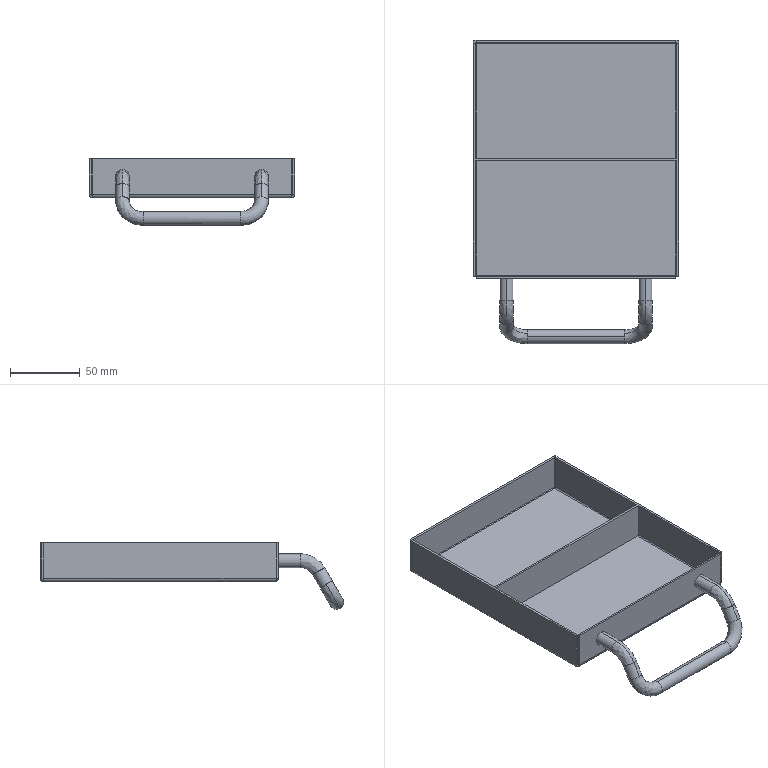Part | STEP file | 02-11 reject box (Default_as machined_) | 2 solids | 105 faces | box 148 x 218 x 48 mm | volume 83489 mm3 | plane 49 | cylinder 30 | spline 18 | cone 8 | commonest cylinder face diameters 1.473 x6 10 x6 4.134 x4 4.473 x4 4.5 x4 9.998 x4